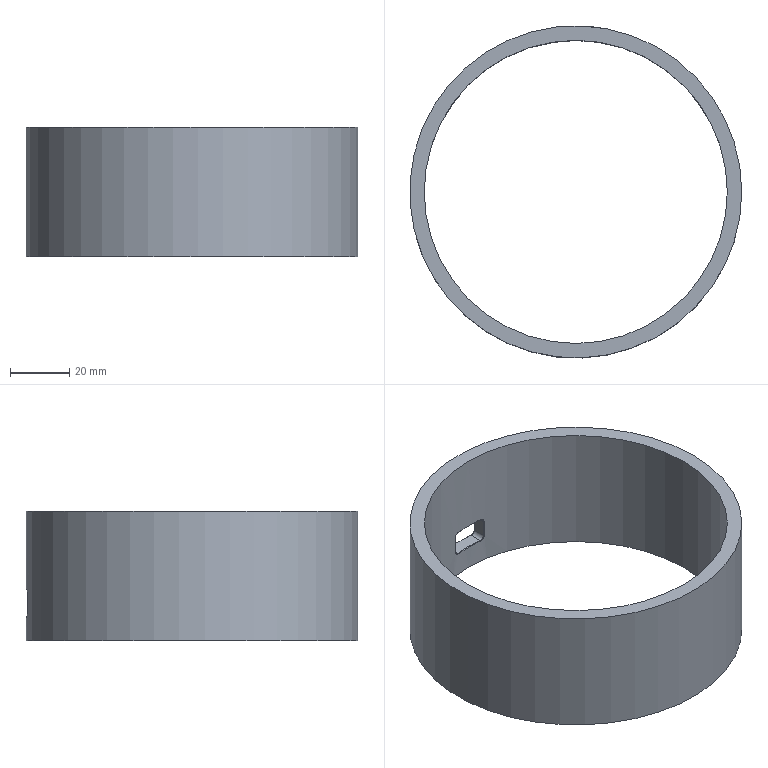CAM job | NX | 3+2 milling | part box 112.5 x 112.5 x 44 mm | stock box 112.5 x 112.5 x 44 mm
Tools:
number,name,description,diameter,corner_radius,flute_length,length,flutes
5,D3,Milling Tool-5 Parameters,3.0,0.0,50.0,75.0,2
7,D6A45,Milling Tool-5 Parameters,6.0,0.0,50.0,75.0,2
6,D4_LOLLIPOP,Spherical Mill,4.0,2.0,3.732,50.0,2
4,D6,Milling Tool-5 Parameters,6.0,0.0,50.0,75.0,2
Operations:
program,operation,operation_type,tool,method,geometry_group,spindle_rpm,surface_speed,feed_per_tooth,feed_cut,feed_plunge,cut_length_mm,path_length_mm,cut_time_min,machine_time_min
1,ZLEVEL_PROFILE_COPY,ZLevelMilling,D6,METHOD,A,9500.0,179.0,0.0789,1500.0,100.0,314.618,377.987,0.2097,0.2161
1,ADAPTIVE_MILLING,CavityMilling,D3,METHOD,A,9500.0,89.0,0.0579,1100.0,100.0,262.457,539.001,0.2386,0.2663
1,ZLEVEL_PROFILE,ZLevelMilling,D3,METHOD,A,9500.0,89.0,0.0632,1200.0,100.0,33.989,106.727,0.0283,0.0356
1,PROFILE_3D,PlanarMilling,D6A45,METHOD,A,9500.0,179.0,0.0658,1250.0,100.0,42.007,102.547,0.0336,0.0397
1,FIXED_CONTOUR,SurfaceContour,D4_LOLLIPOP,METHOD,MCS_MILL,9500.0,179.0,0.0658,1250.0,100.0,46.134,116.475,0.0369,0.0439